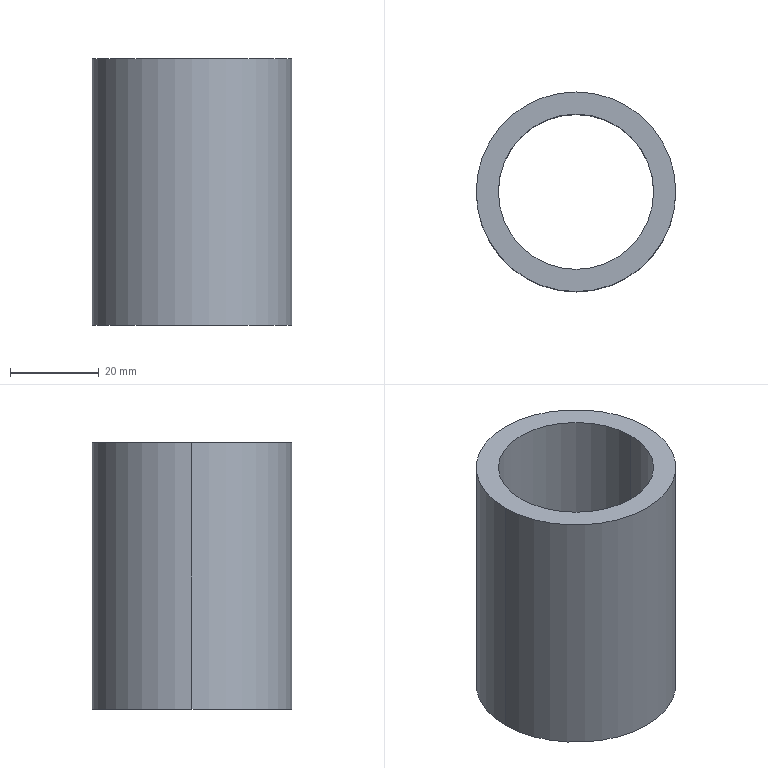Part | SolidWorks | features BaseBody 1 | 1 solid | 6 faces | box 45 x 45 x 60 mm | volume 37699 mm3 | cylinder 4 | plane 2 | commonest cylinder face diameters 35 x2 45 x2
STEP:
#1=CARTESIAN_POINT('',(323.083,269.388,136.922));
#2=VERTEX_POINT('',#1);
#3=CARTESIAN_POINT('',(358.083,269.388,136.922));
#4=VERTEX_POINT('',#3);
#5=CARTESIAN_POINT('',(340.583,269.388,136.922));
#6=DIRECTION('',(0.,0.,-1.));
#7=DIRECTION('',(1.,0.,0.));
#8=AXIS2_PLACEMENT_3D('',#5,#6,#7);
#9=CIRCLE('',#8,17.5);
#10=EDGE_CURVE('',#2,#4,#9,.T.);
#11=ORIENTED_EDGE('',*,*,#10,.F.);
#12=CARTESIAN_POINT('',(323.083,269.388,76.922));
#13=VERTEX_POINT('',#12);
#14=CARTESIAN_POINT('',(323.083,269.388,96.373));
#15=DIRECTION('',(0.,0.,-1.));
#16=VECTOR('',#15,1000.);
#17=LINE('',#14,#16);
#18=EDGE_CURVE('',#2,#13,#17,.T.);
#19=ORIENTED_EDGE('',*,*,#18,.T.);
#20=CARTESIAN_POINT('',(358.083,269.388,76.922));
#21=VERTEX_POINT('',#20);
#22=CARTESIAN_POINT('',(340.583,269.388,76.922));
#23=DIRECTION('',(0.,0.,1.));
#24=DIRECTION('',(1.,0.,0.));
#25=AXIS2_PLACEMENT_3D('',#22,#23,#24);
#26=CIRCLE('',#25,17.5);
#27=EDGE_CURVE('',#21,#13,#26,.T.);
#28=ORIENTED_EDGE('',*,*,#27,.F.);
#29=CARTESIAN_POINT('',(358.083,269.388,96.373));
#30=DIRECTION('',(0.,0.,-1.));
#31=VECTOR('',#30,1000.);
#32=LINE('',#29,#31);
#33=EDGE_CURVE('',#4,#21,#32,.T.);
#34=ORIENTED_EDGE('',*,*,#33,.F.);
#35=EDGE_LOOP('',(#11,#19,#28,#34));
#36=FACE_OUTER_BOUND('',#35,.T.);
#37=CARTESIAN_POINT('',(340.583,269.388,96.373));
#38=DIRECTION('',(0.,0.,-1.));
#39=DIRECTION('',(1.,0.,0.));
#40=AXIS2_PLACEMENT_3D('',#37,#38,#39);
#41=CYLINDRICAL_SURFACE('',#40,17.5);
#42=ADVANCED_FACE('',(#36),#41,.F.);
#43=CARTESIAN_POINT('',(318.083,269.388,136.922));
#44=VERTEX_POINT('',#43);
#45=CARTESIAN_POINT('',(363.083,269.388,136.922));
#46=VERTEX_POINT('',#45);
#47=CARTESIAN_POINT('',(340.583,269.388,136.922));
#48=DIRECTION('',(0.,0.,1.));
#49=DIRECTION('',(-1.,0.,0.));
#50=AXIS2_PLACEMENT_3D('',#47,#48,#49);
#51=CIRCLE('',#50,22.5);
#52=EDGE_CURVE('',#44,#46,#51,.T.);
#53=ORIENTED_EDGE('',*,*,#52,.F.);
#54=CARTESIAN_POINT('',(318.083,269.388,76.922));
#55=VERTEX_POINT('',#54);
#56=CARTESIAN_POINT('',(318.083,269.388,96.373));
#57=DIRECTION('',(0.,0.,-1.));
#58=VECTOR('',#57,1000.);
#59=LINE('',#56,#58);
#60=EDGE_CURVE('',#44,#55,#59,.T.);
#61=ORIENTED_EDGE('',*,*,#60,.T.);
#62=CARTESIAN_POINT('',(363.083,269.388,76.922));
#63=VERTEX_POINT('',#62);
#64=CARTESIAN_POINT('',(340.583,269.388,76.922));
#65=DIRECTION('',(0.,0.,-1.));
#66=DIRECTION('',(1.,0.,0.));
#67=AXIS2_PLACEMENT_3D('',#64,#65,#66);
#68=CIRCLE('',#67,22.5);
#69=EDGE_CURVE('',#63,#55,#68,.T.);
#70=ORIENTED_EDGE('',*,*,#69,.F.);
#71=CARTESIAN_POINT('',(363.083,269.388,96.373));
#72=DIRECTION('',(0.,0.,-1.));
#73=VECTOR('',#72,1000.);
#74=LINE('',#71,#73);
#75=EDGE_CURVE('',#46,#63,#74,.T.);
#76=ORIENTED_EDGE('',*,*,#75,.F.);
#77=EDGE_LOOP('',(#53,#61,#70,#76));
#78=FACE_OUTER_BOUND('',#77,.T.);
#79=CARTESIAN_POINT('',(340.583,269.388,96.373));
#80=DIRECTION('',(0.,0.,-1.));
#81=DIRECTION('',(1.,0.,0.));
#82=AXIS2_PLACEMENT_3D('',#79,#80,#81);
#83=CYLINDRICAL_SURFACE('',#82,22.5);
#84=ADVANCED_FACE('',(#78),#83,.T.);
#85=ORIENTED_EDGE('',*,*,#60,.F.);
#86=CARTESIAN_POINT('',(340.583,269.388,136.922));
#87=DIRECTION('',(0.,0.,1.));
#88=DIRECTION('',(-1.,0.,0.));
#89=AXIS2_PLACEMENT_3D('',#86,#87,#88);
#90=CIRCLE('',#89,22.5);
#91=EDGE_CURVE('',#46,#44,#90,.T.);
#92=ORIENTED_EDGE('',*,*,#91,.F.);
#93=ORIENTED_EDGE('',*,*,#75,.T.);
#94=CARTESIAN_POINT('',(340.583,269.388,76.922));
#95=DIRECTION('',(0.,0.,-1.));
#96=DIRECTION('',(1.,0.,0.));
#97=AXIS2_PLACEMENT_3D('',#94,#95,#96);
#98=CIRCLE('',#97,22.5);
#99=EDGE_CURVE('',#55,#63,#98,.T.);
#100=ORIENTED_EDGE('',*,*,#99,.F.);
#101=EDGE_LOOP('',(#85,#92,#93,#100));
#102=FACE_OUTER_BOUND('',#101,.T.);
#103=CARTESIAN_POINT('',(340.583,269.388,96.373));
#104=DIRECTION('',(0.,0.,-1.));
#105=DIRECTION('',(1.,0.,0.));
#106=AXIS2_PLACEMENT_3D('',#103,#104,#105);
#107=CYLINDRICAL_SURFACE('',#106,22.5);
#108=ADVANCED_FACE('',(#102),#107,.T.);
#109=CARTESIAN_POINT('',(340.583,269.388,136.922));
#110=DIRECTION('',(0.,0.,-1.));
#111=DIRECTION('',(1.,0.,0.));
#112=AXIS2_PLACEMENT_3D('',#109,#110,#111);
#113=CIRCLE('',#112,17.5);
#114=EDGE_CURVE('',#4,#2,#113,.T.);
#115=ORIENTED_EDGE('',*,*,#114,.T.);
#116=ORIENTED_EDGE('',*,*,#10,.T.);
#117=EDGE_LOOP('',(#115,#116));
#118=FACE_BOUND('',#117,.T.);
#119=ORIENTED_EDGE('',*,*,#91,.T.);
#120=ORIENTED_EDGE('',*,*,#52,.T.);
#121=EDGE_LOOP('',(#119,#120));
#122=FACE_OUTER_BOUND('',#121,.T.);
#123=CARTESIAN_POINT('',(324.029,485.948,136.922));
#124=DIRECTION('',(0.,0.,1.));
#125=DIRECTION('',(1.,0.,0.));
#126=AXIS2_PLACEMENT_3D('',#123,#124,#125);
#127=PLANE('',#126);
#128=ADVANCED_FACE('',(#118,#122),#127,.T.);
#129=ORIENTED_EDGE('',*,*,#18,.F.);
#130=ORIENTED_EDGE('',*,*,#114,.F.);
#131=ORIENTED_EDGE('',*,*,#33,.T.);
#132=CARTESIAN_POINT('',(340.583,269.388,76.922));
#133=DIRECTION('',(0.,0.,1.));
#134=DIRECTION('',(1.,0.,0.));
#135=AXIS2_PLACEMENT_3D('',#132,#133,#134);
#136=CIRCLE('',#135,17.5);
#137=EDGE_CURVE('',#13,#21,#136,.T.);
#138=ORIENTED_EDGE('',*,*,#137,.F.);
#139=EDGE_LOOP('',(#129,#130,#131,#138));
#140=FACE_OUTER_BOUND('',#139,.T.);
#141=CARTESIAN_POINT('',(340.583,269.388,96.373));
#142=DIRECTION('',(0.,0.,-1.));
#143=DIRECTION('',(1.,0.,0.));
#144=AXIS2_PLACEMENT_3D('',#141,#142,#143);
#145=CYLINDRICAL_SURFACE('',#144,17.5);
#146=ADVANCED_FACE('',(#140),#145,.F.);
#147=ORIENTED_EDGE('',*,*,#27,.T.);
#148=ORIENTED_EDGE('',*,*,#137,.T.);
#149=EDGE_LOOP('',(#147,#148));
#150=FACE_BOUND('',#149,.T.);
#151=ORIENTED_EDGE('',*,*,#69,.T.);
#152=ORIENTED_EDGE('',*,*,#99,.T.);
#153=EDGE_LOOP('',(#151,#152));
#154=FACE_OUTER_BOUND('',#153,.T.);
#155=CARTESIAN_POINT('',(340.583,269.388,76.922));
#156=DIRECTION('',(0.,0.,-1.));
#157=DIRECTION('',(0.,-1.,0.));
#158=AXIS2_PLACEMENT_3D('',#155,#156,#157);
#159=PLANE('',#158);
#160=ADVANCED_FACE('',(#150,#154),#159,.T.);
#161=CLOSED_SHELL('',(#42,#84,#108,#128,#146,#160));
#162=MANIFOLD_SOLID_BREP('',#161);
#163=CARTESIAN_POINT('',(0.,0.,0.));
#164=DIRECTION('',(0.,0.,1.));
#165=DIRECTION('',(1.,0.,0.));
#166=AXIS2_PLACEMENT_3D('',#163,#164,#165);
#167=(LENGTH_UNIT()NAMED_UNIT(*)SI_UNIT(.MILLI.,.METRE.));
#168=UNCERTAINTY_MEASURE_WITH_UNIT(LENGTH_MEASURE(0.00001),#167,'','');
#169=(NAMED_UNIT(*)PLANE_ANGLE_UNIT()SI_UNIT($,.RADIAN.));
#170=(NAMED_UNIT(*)SI_UNIT($,.STERADIAN.)SOLID_ANGLE_UNIT());
#171=(GEOMETRIC_REPRESENTATION_CONTEXT(3)GLOBAL_UNCERTAINTY_ASSIGNED_CONTEXT((#168))GLOBAL_UNIT_ASSIGNED_CONTEXT((#167,#169,#170))REPRESENTATION_CONTEXT('',''));
#172=ADVANCED_BREP_SHAPE_REPRESENTATION('',(#162,#166),#171);